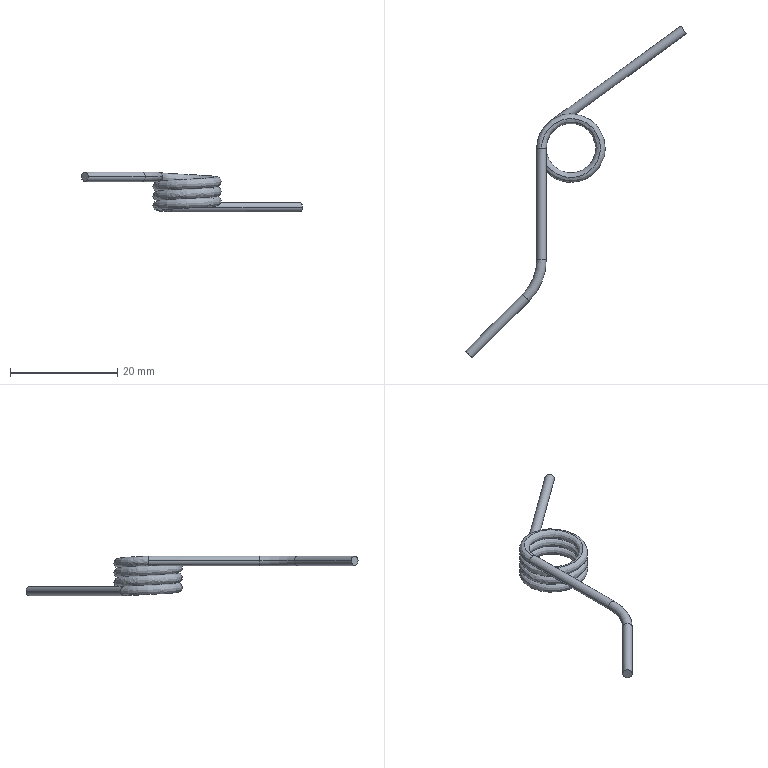Part | NX | features BREP 1 | 1 solid | 12 faces | box 41.247 x 61.989 x 7.45 mm | volume 454.454 mm3 | cylinder 6 | plane 2 | spline 2 | torus 2 | commonest cylinder face diameters 1.78 x6